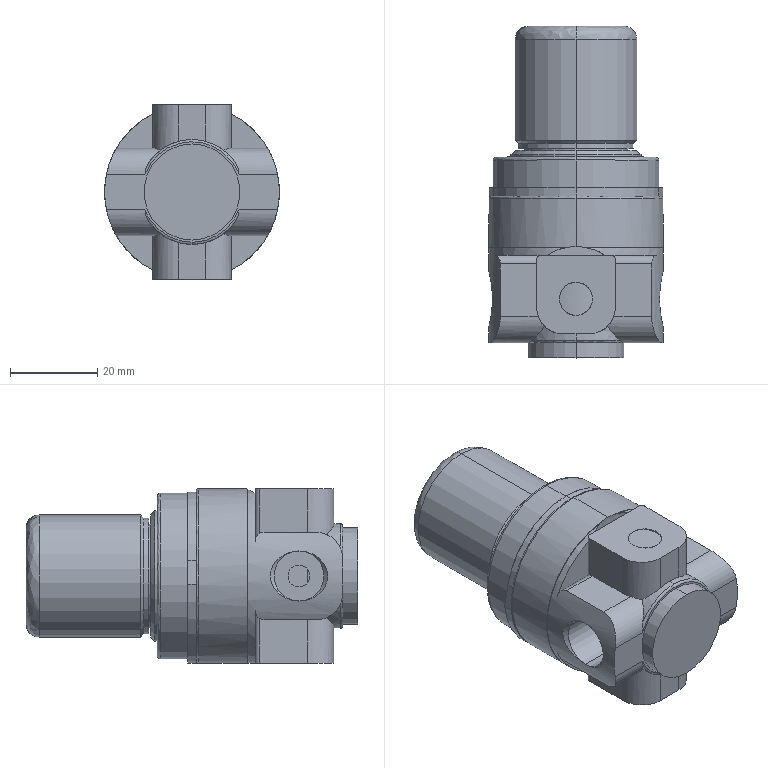Part | 1 solid | 124 faces | box 40 x 76 x 40 mm | volume 65879 mm3 | cylinder 59 | plane 46 | spline 11 | cone 8 | commonest cylinder face diameters 12 x9 24 x8 7.591 x7 40 x5 2 x4 4 x4